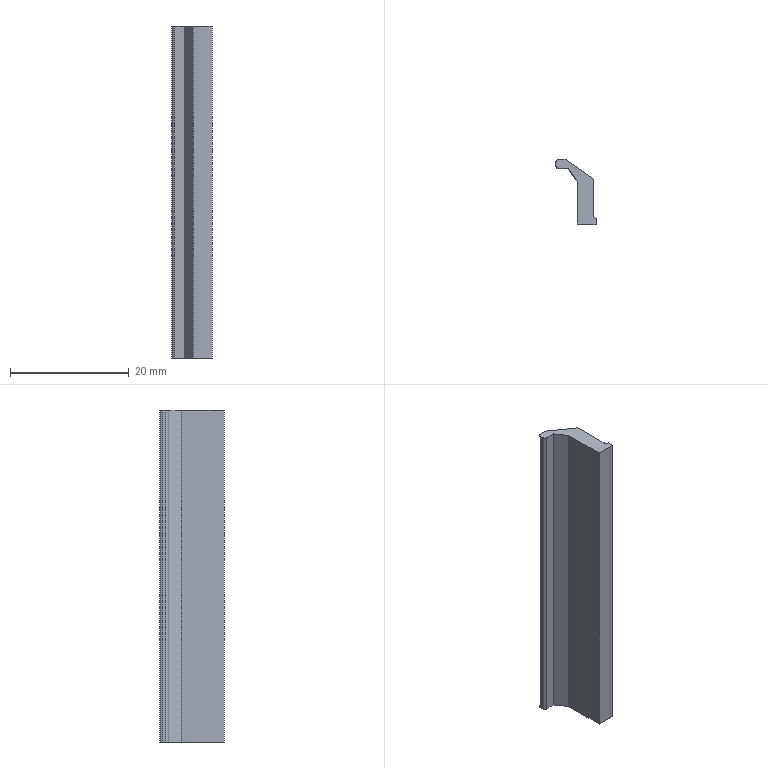Part | NX | features BREP 2 | 2 solids | 32 faces | box 6.787 x 10.9 x 56 mm | volume 3290 mm3 | plane 22 | cylinder 10 | commonest cylinder face diameters 1 x10
STEP:
#1=CARTESIAN_POINT('',(0.2096,1.761,-4.));
#2=VERTEX_POINT('',#1);
#3=CARTESIAN_POINT('',(0.2096,1.761,52.));
#4=VERTEX_POINT('',#3);
#5=CARTESIAN_POINT('',(0.2096,1.761,0.));
#6=DIRECTION('',(0.,0.,1.));
#7=VECTOR('',#6,1000.);
#8=LINE('',#5,#7);
#9=EDGE_CURVE('',#2,#4,#8,.T.);
#10=ORIENTED_EDGE('',*,*,#9,.F.);
#11=CARTESIAN_POINT('',(0.2096,-5.472,-4.));
#12=VERTEX_POINT('',#11);
#13=CARTESIAN_POINT('',(0.2096,24.029,-4.));
#14=DIRECTION('',(0.,-1.,0.));
#15=VECTOR('',#14,1000.);
#16=LINE('',#13,#15);
#17=EDGE_CURVE('',#2,#12,#16,.T.);
#18=ORIENTED_EDGE('',*,*,#17,.T.);
#19=CARTESIAN_POINT('',(0.2096,-5.472,52.));
#20=VERTEX_POINT('',#19);
#21=CARTESIAN_POINT('',(0.2096,-5.472,0.));
#22=DIRECTION('',(0.,0.,1.));
#23=VECTOR('',#22,1000.);
#24=LINE('',#21,#23);
#25=EDGE_CURVE('',#12,#20,#24,.T.);
#26=ORIENTED_EDGE('',*,*,#25,.T.);
#27=CARTESIAN_POINT('',(0.2096,24.029,52.));
#28=DIRECTION('',(0.,-1.,0.));
#29=VECTOR('',#28,1000.);
#30=LINE('',#27,#29);
#31=EDGE_CURVE('',#4,#20,#30,.T.);
#32=ORIENTED_EDGE('',*,*,#31,.F.);
#33=EDGE_LOOP('',(#10,#18,#26,#32));
#34=FACE_BOUND('',#33,.T.);
#35=CARTESIAN_POINT('',(0.2096,-4.473,0.));
#36=DIRECTION('',(1.,0.,0.));
#37=DIRECTION('',(0.,-1.,0.));
#38=AXIS2_PLACEMENT_3D('',#35,#36,#37);
#39=PLANE('',#38);
#40=ADVANCED_FACE('',(#34),#39,.F.);
#41=ORIENTED_EDGE('',*,*,#9,.T.);
#42=CARTESIAN_POINT('',(-1.308,3.928,52.));
#43=VERTEX_POINT('',#42);
#44=CARTESIAN_POINT('',(0.2096,1.761,52.));
#45=DIRECTION('',(0.5736,-0.8192,0.));
#46=VECTOR('',#45,1000.);
#47=LINE('',#44,#46);
#48=EDGE_CURVE('',#43,#4,#47,.T.);
#49=ORIENTED_EDGE('',*,*,#48,.F.);
#50=CARTESIAN_POINT('',(-1.308,3.928,-4.));
#51=VERTEX_POINT('',#50);
#52=CARTESIAN_POINT('',(-1.308,3.928,0.));
#53=DIRECTION('',(0.,0.,1.));
#54=VECTOR('',#53,1000.);
#55=LINE('',#52,#54);
#56=EDGE_CURVE('',#51,#43,#55,.T.);
#57=ORIENTED_EDGE('',*,*,#56,.F.);
#58=CARTESIAN_POINT('',(0.2096,1.761,-4.));
#59=DIRECTION('',(0.5736,-0.8192,0.));
#60=VECTOR('',#59,1000.);
#61=LINE('',#58,#60);
#62=EDGE_CURVE('',#51,#2,#61,.T.);
#63=ORIENTED_EDGE('',*,*,#62,.T.);
#64=EDGE_LOOP('',(#41,#49,#57,#63));
#65=FACE_BOUND('',#64,.T.);
#66=CARTESIAN_POINT('',(0.2096,1.761,0.));
#67=DIRECTION('',(0.8192,0.5736,0.));
#68=DIRECTION('',(0.5736,-0.8192,0.));
#69=AXIS2_PLACEMENT_3D('',#66,#67,#68);
#70=PLANE('',#69);
#71=ADVANCED_FACE('',(#65),#70,.F.);
#72=CARTESIAN_POINT('',(-2.894,3.928,-4.));
#73=VERTEX_POINT('',#72);
#74=CARTESIAN_POINT('',(-2.894,3.928,52.));
#75=VERTEX_POINT('',#74);
#76=CARTESIAN_POINT('',(-2.894,3.928,0.));
#77=DIRECTION('',(0.,0.,1.));
#78=VECTOR('',#77,1000.);
#79=LINE('',#76,#78);
#80=EDGE_CURVE('',#73,#75,#79,.T.);
#81=ORIENTED_EDGE('',*,*,#80,.F.);
#82=CARTESIAN_POINT('',(2.18,3.928,-4.));
#83=DIRECTION('',(1.,0.,0.));
#84=VECTOR('',#83,1000.);
#85=LINE('',#82,#84);
#86=EDGE_CURVE('',#73,#51,#85,.T.);
#87=ORIENTED_EDGE('',*,*,#86,.T.);
#88=ORIENTED_EDGE('',*,*,#56,.T.);
#89=CARTESIAN_POINT('',(2.18,3.928,52.));
#90=DIRECTION('',(1.,0.,0.));
#91=VECTOR('',#90,1000.);
#92=LINE('',#89,#91);
#93=EDGE_CURVE('',#75,#43,#92,.T.);
#94=ORIENTED_EDGE('',*,*,#93,.F.);
#95=EDGE_LOOP('',(#81,#87,#88,#94));
#96=FACE_BOUND('',#95,.T.);
#97=CARTESIAN_POINT('',(-2.694,3.928,0.));
#98=DIRECTION('',(0.,1.,0.));
#99=DIRECTION('',(1.,0.,0.));
#100=AXIS2_PLACEMENT_3D('',#97,#98,#99);
#101=PLANE('',#100);
#102=ADVANCED_FACE('',(#96),#101,.F.);
#103=ORIENTED_EDGE('',*,*,#80,.T.);
#104=CARTESIAN_POINT('',(-3.394,4.428,52.));
#105=VERTEX_POINT('',#104);
#106=CARTESIAN_POINT('',(-2.894,4.428,52.));
#107=DIRECTION('',(0.,0.,1.));
#108=DIRECTION('',(1.,0.,0.));
#109=AXIS2_PLACEMENT_3D('',#106,#107,#108);
#110=CIRCLE('',#109,0.5);
#111=EDGE_CURVE('',#105,#75,#110,.T.);
#112=ORIENTED_EDGE('',*,*,#111,.F.);
#113=CARTESIAN_POINT('',(-3.394,4.428,-4.));
#114=VERTEX_POINT('',#113);
#115=CARTESIAN_POINT('',(-3.394,4.428,0.));
#116=DIRECTION('',(0.,0.,1.));
#117=VECTOR('',#116,1000.);
#118=LINE('',#115,#117);
#119=EDGE_CURVE('',#114,#105,#118,.T.);
#120=ORIENTED_EDGE('',*,*,#119,.F.);
#121=CARTESIAN_POINT('',(-2.894,4.428,-4.));
#122=DIRECTION('',(0.,0.,1.));
#123=DIRECTION('',(1.,0.,0.));
#124=AXIS2_PLACEMENT_3D('',#121,#122,#123);
#125=CIRCLE('',#124,0.5);
#126=EDGE_CURVE('',#114,#73,#125,.T.);
#127=ORIENTED_EDGE('',*,*,#126,.T.);
#128=EDGE_LOOP('',(#103,#112,#120,#127));
#129=FACE_BOUND('',#128,.T.);
#130=CARTESIAN_POINT('',(-2.894,4.428,0.));
#131=DIRECTION('',(0.,0.,1.));
#132=DIRECTION('',(-1.,0.,0.));
#133=AXIS2_PLACEMENT_3D('',#130,#131,#132);
#134=CYLINDRICAL_SURFACE('',#133,0.5);
#135=ADVANCED_FACE('',(#129),#134,.T.);
#136=ORIENTED_EDGE('',*,*,#119,.T.);
#137=CARTESIAN_POINT('',(-3.394,4.928,52.));
#138=VERTEX_POINT('',#137);
#139=CARTESIAN_POINT('',(-3.394,24.029,52.));
#140=DIRECTION('',(0.,-1.,0.));
#141=VECTOR('',#140,1000.);
#142=LINE('',#139,#141);
#143=EDGE_CURVE('',#138,#105,#142,.T.);
#144=ORIENTED_EDGE('',*,*,#143,.F.);
#145=CARTESIAN_POINT('',(-3.394,4.928,-4.));
#146=VERTEX_POINT('',#145);
#147=CARTESIAN_POINT('',(-3.394,4.928,0.));
#148=DIRECTION('',(0.,0.,1.));
#149=VECTOR('',#148,1000.);
#150=LINE('',#147,#149);
#151=EDGE_CURVE('',#146,#138,#150,.T.);
#152=ORIENTED_EDGE('',*,*,#151,.F.);
#153=CARTESIAN_POINT('',(-3.394,24.029,-4.));
#154=DIRECTION('',(0.,-1.,0.));
#155=VECTOR('',#154,1000.);
#156=LINE('',#153,#155);
#157=EDGE_CURVE('',#146,#114,#156,.T.);
#158=ORIENTED_EDGE('',*,*,#157,.T.);
#159=EDGE_LOOP('',(#136,#144,#152,#158));
#160=FACE_BOUND('',#159,.T.);
#161=CARTESIAN_POINT('',(-3.394,4.428,0.));
#162=DIRECTION('',(1.,0.,0.));
#163=DIRECTION('',(0.,-1.,0.));
#164=AXIS2_PLACEMENT_3D('',#161,#162,#163);
#165=PLANE('',#164);
#166=ADVANCED_FACE('',(#160),#165,.F.);
#167=ORIENTED_EDGE('',*,*,#151,.T.);
#168=CARTESIAN_POINT('',(-2.894,5.428,52.));
#169=VERTEX_POINT('',#168);
#170=CARTESIAN_POINT('',(-2.894,4.928,52.));
#171=DIRECTION('',(0.,0.,1.));
#172=DIRECTION('',(1.,0.,0.));
#173=AXIS2_PLACEMENT_3D('',#170,#171,#172);
#174=CIRCLE('',#173,0.5);
#175=EDGE_CURVE('',#169,#138,#174,.T.);
#176=ORIENTED_EDGE('',*,*,#175,.F.);
#177=CARTESIAN_POINT('',(-2.894,5.428,-4.));
#178=VERTEX_POINT('',#177);
#179=CARTESIAN_POINT('',(-2.894,5.427,0.));
#180=DIRECTION('',(0.,0.,1.));
#181=VECTOR('',#180,1000.);
#182=LINE('',#179,#181);
#183=EDGE_CURVE('',#178,#169,#182,.T.);
#184=ORIENTED_EDGE('',*,*,#183,.F.);
#185=CARTESIAN_POINT('',(-2.894,4.928,-4.));
#186=DIRECTION('',(0.,0.,1.));
#187=DIRECTION('',(1.,0.,0.));
#188=AXIS2_PLACEMENT_3D('',#185,#186,#187);
#189=CIRCLE('',#188,0.5);
#190=EDGE_CURVE('',#178,#146,#189,.T.);
#191=ORIENTED_EDGE('',*,*,#190,.T.);
#192=EDGE_LOOP('',(#167,#176,#184,#191));
#193=FACE_BOUND('',#192,.T.);
#194=CARTESIAN_POINT('',(-2.894,4.928,0.));
#195=DIRECTION('',(0.,0.,1.));
#196=DIRECTION('',(-1.,0.,0.));
#197=AXIS2_PLACEMENT_3D('',#194,#195,#196);
#198=CYLINDRICAL_SURFACE('',#197,0.5);
#199=ADVANCED_FACE('',(#193),#198,.T.);
#200=ORIENTED_EDGE('',*,*,#183,.T.);
#201=CARTESIAN_POINT('',(-1.851,5.428,52.));
#202=VERTEX_POINT('',#201);
#203=CARTESIAN_POINT('',(2.18,5.427,52.));
#204=DIRECTION('',(-1.,0.,0.));
#205=VECTOR('',#204,1000.);
#206=LINE('',#203,#205);
#207=EDGE_CURVE('',#202,#169,#206,.T.);
#208=ORIENTED_EDGE('',*,*,#207,.F.);
#209=CARTESIAN_POINT('',(-1.851,5.428,-4.));
#210=VERTEX_POINT('',#209);
#211=CARTESIAN_POINT('',(-1.851,5.428,0.));
#212=DIRECTION('',(0.,0.,1.));
#213=VECTOR('',#212,1000.);
#214=LINE('',#211,#213);
#215=EDGE_CURVE('',#210,#202,#214,.T.);
#216=ORIENTED_EDGE('',*,*,#215,.F.);
#217=CARTESIAN_POINT('',(2.18,5.427,-4.));
#218=DIRECTION('',(-1.,0.,0.));
#219=VECTOR('',#218,1000.);
#220=LINE('',#217,#219);
#221=EDGE_CURVE('',#210,#178,#220,.T.);
#222=ORIENTED_EDGE('',*,*,#221,.T.);
#223=EDGE_LOOP('',(#200,#208,#216,#222));
#224=FACE_BOUND('',#223,.T.);
#225=CARTESIAN_POINT('',(-2.894,5.427,0.));
#226=DIRECTION('',(0.,-1.,0.));
#227=DIRECTION('',(-1.,0.,0.));
#228=AXIS2_PLACEMENT_3D('',#225,#226,#227);
#229=PLANE('',#228);
#230=ADVANCED_FACE('',(#224),#229,.F.);
#231=ORIENTED_EDGE('',*,*,#215,.T.);
#232=CARTESIAN_POINT('',(-1.564,5.337,52.));
#233=VERTEX_POINT('',#232);
#234=CARTESIAN_POINT('',(-1.851,4.928,52.));
#235=DIRECTION('',(0.,0.,1.));
#236=DIRECTION('',(1.,0.,0.));
#237=AXIS2_PLACEMENT_3D('',#234,#235,#236);
#238=CIRCLE('',#237,0.5);
#239=EDGE_CURVE('',#233,#202,#238,.T.);
#240=ORIENTED_EDGE('',*,*,#239,.F.);
#241=CARTESIAN_POINT('',(-1.564,5.337,-4.));
#242=VERTEX_POINT('',#241);
#243=CARTESIAN_POINT('',(-1.564,5.337,0.));
#244=DIRECTION('',(0.,0.,1.));
#245=VECTOR('',#244,1000.);
#246=LINE('',#243,#245);
#247=EDGE_CURVE('',#242,#233,#246,.T.);
#248=ORIENTED_EDGE('',*,*,#247,.F.);
#249=CARTESIAN_POINT('',(-1.851,4.928,-4.));
#250=DIRECTION('',(0.,0.,1.));
#251=DIRECTION('',(1.,0.,0.));
#252=AXIS2_PLACEMENT_3D('',#249,#250,#251);
#253=CIRCLE('',#252,0.5);
#254=EDGE_CURVE('',#242,#210,#253,.T.);
#255=ORIENTED_EDGE('',*,*,#254,.T.);
#256=EDGE_LOOP('',(#231,#240,#248,#255));
#257=FACE_BOUND('',#256,.T.);
#258=CARTESIAN_POINT('',(-1.851,4.928,0.));
#259=DIRECTION('',(0.,0.,1.));
#260=DIRECTION('',(-1.,0.,0.));
#261=AXIS2_PLACEMENT_3D('',#258,#259,#260);
#262=CYLINDRICAL_SURFACE('',#261,0.5);
#263=ADVANCED_FACE('',(#257),#262,.T.);
#264=ORIENTED_EDGE('',*,*,#247,.T.);
#265=CARTESIAN_POINT('',(2.68,2.365,52.));
#266=VERTEX_POINT('',#265);
#267=CARTESIAN_POINT('',(-1.564,5.337,52.));
#268=DIRECTION('',(-0.8192,0.5736,0.));
#269=VECTOR('',#268,1000.);
#270=LINE('',#267,#269);
#271=EDGE_CURVE('',#266,#233,#270,.T.);
#272=ORIENTED_EDGE('',*,*,#271,.F.);
#273=CARTESIAN_POINT('',(2.68,2.365,-4.));
#274=VERTEX_POINT('',#273);
#275=CARTESIAN_POINT('',(2.68,2.365,0.));
#276=DIRECTION('',(0.,0.,1.));
#277=VECTOR('',#276,1000.);
#278=LINE('',#275,#277);
#279=EDGE_CURVE('',#274,#266,#278,.T.);
#280=ORIENTED_EDGE('',*,*,#279,.F.);
#281=CARTESIAN_POINT('',(-1.564,5.337,-4.));
#282=DIRECTION('',(-0.8192,0.5736,0.));
#283=VECTOR('',#282,1000.);
#284=LINE('',#281,#283);
#285=EDGE_CURVE('',#274,#242,#284,.T.);
#286=ORIENTED_EDGE('',*,*,#285,.T.);
#287=EDGE_LOOP('',(#264,#272,#280,#286));
#288=FACE_BOUND('',#287,.T.);
#289=CARTESIAN_POINT('',(-1.564,5.337,0.));
#290=DIRECTION('',(-0.5736,-0.8192,0.));
#291=DIRECTION('',(-0.8192,0.5736,0.));
#292=AXIS2_PLACEMENT_3D('',#289,#290,#291);
#293=PLANE('',#292);
#294=ADVANCED_FACE('',(#288),#293,.F.);
#295=ORIENTED_EDGE('',*,*,#279,.T.);
#296=CARTESIAN_POINT('',(2.894,1.955,52.));
#297=VERTEX_POINT('',#296);
#298=CARTESIAN_POINT('',(2.394,1.955,52.));
#299=DIRECTION('',(0.,0.,1.));
#300=DIRECTION('',(1.,0.,0.));
#301=AXIS2_PLACEMENT_3D('',#298,#299,#300);
#302=CIRCLE('',#301,0.5);
#303=EDGE_CURVE('',#297,#266,#302,.T.);
#304=ORIENTED_EDGE('',*,*,#303,.F.);
#305=CARTESIAN_POINT('',(2.894,1.955,-4.));
#306=VERTEX_POINT('',#305);
#307=CARTESIAN_POINT('',(2.894,1.955,0.));
#308=DIRECTION('',(0.,0.,1.));
#309=VECTOR('',#308,1000.);
#310=LINE('',#307,#309);
#311=EDGE_CURVE('',#306,#297,#310,.T.);
#312=ORIENTED_EDGE('',*,*,#311,.F.);
#313=CARTESIAN_POINT('',(2.394,1.955,-4.));
#314=DIRECTION('',(0.,0.,1.));
#315=DIRECTION('',(1.,0.,0.));
#316=AXIS2_PLACEMENT_3D('',#313,#314,#315);
#317=CIRCLE('',#316,0.5);
#318=EDGE_CURVE('',#306,#274,#317,.T.);
#319=ORIENTED_EDGE('',*,*,#318,.T.);
#320=EDGE_LOOP('',(#295,#304,#312,#319));
#321=FACE_BOUND('',#320,.T.);
#322=CARTESIAN_POINT('',(2.394,1.955,0.));
#323=DIRECTION('',(0.,0.,1.));
#324=DIRECTION('',(-1.,0.,0.));
#325=AXIS2_PLACEMENT_3D('',#322,#323,#324);
#326=CYLINDRICAL_SURFACE('',#325,0.5);
#327=ADVANCED_FACE('',(#321),#326,.T.);
#328=ORIENTED_EDGE('',*,*,#311,.T.);
#329=CARTESIAN_POINT('',(2.894,-3.973,52.));
#330=VERTEX_POINT('',#329);
#331=CARTESIAN_POINT('',(2.894,24.029,52.));
#332=DIRECTION('',(0.,1.,0.));
#333=VECTOR('',#332,1000.);
#334=LINE('',#331,#333);
#335=EDGE_CURVE('',#330,#297,#334,.T.);
#336=ORIENTED_EDGE('',*,*,#335,.F.);
#337=CARTESIAN_POINT('',(2.894,-3.973,-4.));
#338=VERTEX_POINT('',#337);
#339=CARTESIAN_POINT('',(2.894,-3.973,0.));
#340=DIRECTION('',(0.,0.,1.));
#341=VECTOR('',#340,1000.);
#342=LINE('',#339,#341);
#343=EDGE_CURVE('',#338,#330,#342,.T.);
#344=ORIENTED_EDGE('',*,*,#343,.F.);
#345=CARTESIAN_POINT('',(2.894,24.029,-4.));
#346=DIRECTION('',(0.,1.,0.));
#347=VECTOR('',#346,1000.);
#348=LINE('',#345,#347);
#349=EDGE_CURVE('',#338,#306,#348,.T.);
#350=ORIENTED_EDGE('',*,*,#349,.T.);
#351=EDGE_LOOP('',(#328,#336,#344,#350));
#352=FACE_BOUND('',#351,.T.);
#353=CARTESIAN_POINT('',(2.894,1.955,0.));
#354=DIRECTION('',(-1.,0.,0.));
#355=DIRECTION('',(0.,1.,0.));
#356=AXIS2_PLACEMENT_3D('',#353,#354,#355);
#357=PLANE('',#356);
#358=ADVANCED_FACE('',(#352),#357,.F.);
#359=ORIENTED_EDGE('',*,*,#343,.T.);
#360=CARTESIAN_POINT('',(3.394,-4.473,52.));
#361=VERTEX_POINT('',#360);
#362=CARTESIAN_POINT('',(3.394,-3.973,52.));
#363=DIRECTION('',(0.,0.,-1.));
#364=DIRECTION('',(1.,0.,0.));
#365=AXIS2_PLACEMENT_3D('',#362,#363,#364);
#366=CIRCLE('',#365,0.5);
#367=EDGE_CURVE('',#361,#330,#366,.T.);
#368=ORIENTED_EDGE('',*,*,#367,.F.);
#369=CARTESIAN_POINT('',(3.394,-4.473,-4.));
#370=VERTEX_POINT('',#369);
#371=CARTESIAN_POINT('',(3.394,-4.473,0.));
#372=DIRECTION('',(0.,0.,1.));
#373=VECTOR('',#372,1000.);
#374=LINE('',#371,#373);
#375=EDGE_CURVE('',#370,#361,#374,.T.);
#376=ORIENTED_EDGE('',*,*,#375,.F.);
#377=CARTESIAN_POINT('',(3.394,-3.973,-4.));
#378=DIRECTION('',(0.,0.,-1.));
#379=DIRECTION('',(1.,0.,0.));
#380=AXIS2_PLACEMENT_3D('',#377,#378,#379);
#381=CIRCLE('',#380,0.5);
#382=EDGE_CURVE('',#370,#338,#381,.T.);
#383=ORIENTED_EDGE('',*,*,#382,.T.);
#384=EDGE_LOOP('',(#359,#368,#376,#383));
#385=FACE_BOUND('',#384,.T.);
#386=CARTESIAN_POINT('',(3.394,-3.973,0.));
#387=DIRECTION('',(0.,0.,1.));
#388=DIRECTION('',(-1.,0.,0.));
#389=AXIS2_PLACEMENT_3D('',#386,#387,#388);
#390=CYLINDRICAL_SURFACE('',#389,0.5);
#391=ADVANCED_FACE('',(#385),#390,.F.);
#392=ORIENTED_EDGE('',*,*,#375,.T.);
#393=CARTESIAN_POINT('',(3.394,-5.472,52.));
#394=VERTEX_POINT('',#393);
#395=CARTESIAN_POINT('',(3.394,24.029,52.));
#396=DIRECTION('',(0.,1.,0.));
#397=VECTOR('',#396,1000.);
#398=LINE('',#395,#397);
#399=EDGE_CURVE('',#394,#361,#398,.T.);
#400=ORIENTED_EDGE('',*,*,#399,.F.);
#401=CARTESIAN_POINT('',(3.394,-5.472,-4.));
#402=VERTEX_POINT('',#401);
#403=CARTESIAN_POINT('',(3.394,-5.473,0.));
#404=DIRECTION('',(0.,0.,1.));
#405=VECTOR('',#404,1000.);
#406=LINE('',#403,#405);
#407=EDGE_CURVE('',#402,#394,#406,.T.);
#408=ORIENTED_EDGE('',*,*,#407,.F.);
#409=CARTESIAN_POINT('',(3.394,24.029,-4.));
#410=DIRECTION('',(0.,1.,0.));
#411=VECTOR('',#410,1000.);
#412=LINE('',#409,#411);
#413=EDGE_CURVE('',#402,#370,#412,.T.);
#414=ORIENTED_EDGE('',*,*,#413,.T.);
#415=EDGE_LOOP('',(#392,#400,#408,#414));
#416=FACE_BOUND('',#415,.T.);
#417=CARTESIAN_POINT('',(3.394,-4.473,0.));
#418=DIRECTION('',(-1.,0.,0.));
#419=DIRECTION('',(0.,1.,0.));
#420=AXIS2_PLACEMENT_3D('',#417,#418,#419);
#421=PLANE('',#420);
#422=ADVANCED_FACE('',(#416),#421,.F.);
#423=CARTESIAN_POINT('',(2.18,-5.472,-4.));
#424=DIRECTION('',(1.,0.,0.));
#425=VECTOR('',#424,1000.);
#426=LINE('',#423,#425);
#427=EDGE_CURVE('',#12,#402,#426,.T.);
#428=ORIENTED_EDGE('',*,*,#427,.T.);
#429=ORIENTED_EDGE('',*,*,#407,.T.);
#430=CARTESIAN_POINT('',(2.18,-5.472,52.));
#431=DIRECTION('',(1.,0.,0.));
#432=VECTOR('',#431,1000.);
#433=LINE('',#430,#432);
#434=EDGE_CURVE('',#20,#394,#433,.T.);
#435=ORIENTED_EDGE('',*,*,#434,.F.);
#436=ORIENTED_EDGE('',*,*,#25,.F.);
#437=EDGE_LOOP('',(#428,#429,#435,#436));
#438=FACE_BOUND('',#437,.T.);
#439=CARTESIAN_POINT('',(0.2096,-5.472,0.));
#440=DIRECTION('',(0.,-1.,0.));
#441=DIRECTION('',(-1.,0.,0.));
#442=AXIS2_PLACEMENT_3D('',#439,#440,#441);
#443=PLANE('',#442);
#444=ADVANCED_FACE('',(#438),#443,.T.);
#445=ORIENTED_EDGE('',*,*,#399,.T.);
#446=ORIENTED_EDGE('',*,*,#367,.T.);
#447=ORIENTED_EDGE('',*,*,#335,.T.);
#448=ORIENTED_EDGE('',*,*,#303,.T.);
#449=ORIENTED_EDGE('',*,*,#271,.T.);
#450=ORIENTED_EDGE('',*,*,#239,.T.);
#451=ORIENTED_EDGE('',*,*,#207,.T.);
#452=ORIENTED_EDGE('',*,*,#175,.T.);
#453=ORIENTED_EDGE('',*,*,#143,.T.);
#454=ORIENTED_EDGE('',*,*,#111,.T.);
#455=ORIENTED_EDGE('',*,*,#93,.T.);
#456=ORIENTED_EDGE('',*,*,#48,.T.);
#457=ORIENTED_EDGE('',*,*,#31,.T.);
#458=ORIENTED_EDGE('',*,*,#434,.T.);
#459=EDGE_LOOP('',(#445,#446,#447,#448,#449,#450,#451,#452,#453,#454,#455,#456,#457,#458));
#460=FACE_BOUND('',#459,.T.);
#461=CARTESIAN_POINT('',(2.18,24.029,52.));
#462=DIRECTION('',(0.,0.,1.));
#463=DIRECTION('',(-1.,0.,0.));
#464=AXIS2_PLACEMENT_3D('',#461,#462,#463);
#465=PLANE('',#464);
#466=ADVANCED_FACE('',(#460),#465,.T.);
#467=ORIENTED_EDGE('',*,*,#413,.F.);
#468=ORIENTED_EDGE('',*,*,#427,.F.);
#469=ORIENTED_EDGE('',*,*,#17,.F.);
#470=ORIENTED_EDGE('',*,*,#62,.F.);
#471=ORIENTED_EDGE('',*,*,#86,.F.);
#472=ORIENTED_EDGE('',*,*,#126,.F.);
#473=ORIENTED_EDGE('',*,*,#157,.F.);
#474=ORIENTED_EDGE('',*,*,#190,.F.);
#475=ORIENTED_EDGE('',*,*,#221,.F.);
#476=ORIENTED_EDGE('',*,*,#254,.F.);
#477=ORIENTED_EDGE('',*,*,#285,.F.);
#478=ORIENTED_EDGE('',*,*,#318,.F.);
#479=ORIENTED_EDGE('',*,*,#349,.F.);
#480=ORIENTED_EDGE('',*,*,#382,.F.);
#481=EDGE_LOOP('',(#467,#468,#469,#470,#471,#472,#473,#474,#475,#476,#477,#478,#479,#480));
#482=FACE_BOUND('',#481,.T.);
#483=CARTESIAN_POINT('',(2.18,24.029,-4.));
#484=DIRECTION('',(0.,0.,1.));
#485=DIRECTION('',(-1.,0.,0.));
#486=AXIS2_PLACEMENT_3D('',#483,#484,#485);
#487=PLANE('',#486);
#488=ADVANCED_FACE('',(#482),#487,.F.);
#489=CLOSED_SHELL('',(#40,#71,#102,#135,#166,#199,#230,#263,#294,#327,#358,#391,#422,#444,#466,#488));
#490=MANIFOLD_SOLID_BREP('',#489);
#491=CARTESIAN_POINT('',(0.2096,1.761,-4.));
#492=VERTEX_POINT('',#491);
#493=CARTESIAN_POINT('',(0.2096,1.761,52.));
#494=VERTEX_POINT('',#493);
#495=CARTESIAN_POINT('',(0.2096,1.761,0.));
#496=DIRECTION('',(0.,0.,1.));
#497=VECTOR('',#496,1000.);
#498=LINE('',#495,#497);
#499=EDGE_CURVE('',#492,#494,#498,.T.);
#500=ORIENTED_EDGE('',*,*,#499,.F.);
#501=CARTESIAN_POINT('',(0.2096,-5.472,-4.));
#502=VERTEX_POINT('',#501);
#503=CARTESIAN_POINT('',(0.2096,24.029,-4.));
#504=DIRECTION('',(0.,-1.,0.));
#505=VECTOR('',#504,1000.);
#506=LINE('',#503,#505);
#507=EDGE_CURVE('',#492,#502,#506,.T.);
#508=ORIENTED_EDGE('',*,*,#507,.T.);
#509=CARTESIAN_POINT('',(0.2096,-5.472,52.));
#510=VERTEX_POINT('',#509);
#511=CARTESIAN_POINT('',(0.2096,-5.472,0.));
#512=DIRECTION('',(0.,0.,1.));
#513=VECTOR('',#512,1000.);
#514=LINE('',#511,#513);
#515=EDGE_CURVE('',#502,#510,#514,.T.);
#516=ORIENTED_EDGE('',*,*,#515,.T.);
#517=CARTESIAN_POINT('',(0.2096,24.029,52.));
#518=DIRECTION('',(0.,-1.,0.));
#519=VECTOR('',#518,1000.);
#520=LINE('',#517,#519);
#521=EDGE_CURVE('',#494,#510,#520,.T.);
#522=ORIENTED_EDGE('',*,*,#521,.F.);
#523=EDGE_LOOP('',(#500,#508,#516,#522));
#524=FACE_BOUND('',#523,.T.);
#525=CARTESIAN_POINT('',(0.2096,-4.473,0.));
#526=DIRECTION('',(1.,0.,0.));
#527=DIRECTION('',(0.,-1.,0.));
#528=AXIS2_PLACEMENT_3D('',#525,#526,#527);
#529=PLANE('',#528);
#530=ADVANCED_FACE('',(#524),#529,.F.);
#531=ORIENTED_EDGE('',*,*,#499,.T.);
#532=CARTESIAN_POINT('',(-1.308,3.928,52.));
#533=VERTEX_POINT('',#532);
#534=CARTESIAN_POINT('',(0.2096,1.761,52.));
#535=DIRECTION('',(0.5736,-0.8192,0.));
#536=VECTOR('',#535,1000.);
#537=LINE('',#534,#536);
#538=EDGE_CURVE('',#533,#494,#537,.T.);
#539=ORIENTED_EDGE('',*,*,#538,.F.);
#540=CARTESIAN_POINT('',(-1.308,3.928,-4.));
#541=VERTEX_POINT('',#540);
#542=CARTESIAN_POINT('',(-1.308,3.928,0.));
#543=DIRECTION('',(0.,0.,1.));
#544=VECTOR('',#543,1000.);
#545=LINE('',#542,#544);
#546=EDGE_CURVE('',#541,#533,#545,.T.);
#547=ORIENTED_EDGE('',*,*,#546,.F.);
#548=CARTESIAN_POINT('',(0.2096,1.761,-4.));
#549=DIRECTION('',(0.5736,-0.8192,0.));
#550=VECTOR('',#549,1000.);
#551=LINE('',#548,#550);
#552=EDGE_CURVE('',#541,#492,#551,.T.);
#553=ORIENTED_EDGE('',*,*,#552,.T.);
#554=EDGE_LOOP('',(#531,#539,#547,#553));
#555=FACE_BOUND('',#554,.T.);
#556=CARTESIAN_POINT('',(0.2096,1.761,0.));
#557=DIRECTION('',(0.8192,0.5736,0.));
#558=DIRECTION('',(0.5736,-0.8192,0.));
#559=AXIS2_PLACEMENT_3D('',#556,#557,#558);
#560=PLANE('',#559);
#561=ADVANCED_FACE('',(#555),#560,.F.);
#562=CARTESIAN_POINT('',(-2.894,3.928,-4.));
#563=VERTEX_POINT('',#562);
#564=CARTESIAN_POINT('',(-2.894,3.928,52.));
#565=VERTEX_POINT('',#564);
#566=CARTESIAN_POINT('',(-2.894,3.928,0.));
#567=DIRECTION('',(0.,0.,1.));
#568=VECTOR('',#567,1000.);
#569=LINE('',#566,#568);
#570=EDGE_CURVE('',#563,#565,#569,.T.);
#571=ORIENTED_EDGE('',*,*,#570,.F.);
#572=CARTESIAN_POINT('',(2.18,3.928,-4.));
#573=DIRECTION('',(1.,0.,0.));
#574=VECTOR('',#573,1000.);
#575=LINE('',#572,#574);
#576=EDGE_CURVE('',#563,#541,#575,.T.);
#577=ORIENTED_EDGE('',*,*,#576,.T.);
#578=ORIENTED_EDGE('',*,*,#546,.T.);
#579=CARTESIAN_POINT('',(2.18,3.928,52.));
#580=DIRECTION('',(1.,0.,0.));
#581=VECTOR('',#580,1000.);
#582=LINE('',#579,#581);
#583=EDGE_CURVE('',#565,#533,#582,.T.);
#584=ORIENTED_EDGE('',*,*,#583,.F.);
#585=EDGE_LOOP('',(#571,#577,#578,#584));
#586=FACE_BOUND('',#585,.T.);
#587=CARTESIAN_POINT('',(-2.694,3.928,0.));
#588=DIRECTION('',(0.,1.,0.));
#589=DIRECTION('',(1.,0.,0.));
#590=AXIS2_PLACEMENT_3D('',#587,#588,#589);
#591=PLANE('',#590);
#592=ADVANCED_FACE('',(#586),#591,.F.);
#593=ORIENTED_EDGE('',*,*,#570,.T.);
#594=CARTESIAN_POINT('',(-3.394,4.428,52.));
#595=VERTEX_POINT('',#594);
#596=CARTESIAN_POINT('',(-2.894,4.428,52.));
#597=DIRECTION('',(0.,0.,1.));
#598=DIRECTION('',(1.,0.,0.));
#599=AXIS2_PLACEMENT_3D('',#596,#597,#598);
#600=CIRCLE('',#599,0.5);
#601=EDGE_CURVE('',#595,#565,#600,.T.);
#602=ORIENTED_EDGE('',*,*,#601,.F.);
#603=CARTESIAN_POINT('',(-3.394,4.428,-4.));
#604=VERTEX_POINT('',#603);
#605=CARTESIAN_POINT('',(-3.394,4.428,0.));
#606=DIRECTION('',(0.,0.,1.));
#607=VECTOR('',#606,1000.);
#608=LINE('',#605,#607);
#609=EDGE_CURVE('',#604,#595,#608,.T.);
#610=ORIENTED_EDGE('',*,*,#609,.F.);
#611=CARTESIAN_POINT('',(-2.894,4.428,-4.));
#612=DIRECTION('',(0.,0.,1.));
#613=DIRECTION('',(1.,0.,0.));
#614=AXIS2_PLACEMENT_3D('',#611,#612,#613);
#615=CIRCLE('',#614,0.5);
#616=EDGE_CURVE('',#604,#563,#615,.T.);
#617=ORIENTED_EDGE('',*,*,#616,.T.);
#618=EDGE_LOOP('',(#593,#602,#610,#617));
#619=FACE_BOUND('',#618,.T.);
#620=CARTESIAN_POINT('',(-2.894,4.428,0.));
#621=DIRECTION('',(0.,0.,1.));
#622=DIRECTION('',(-1.,0.,0.));
#623=AXIS2_PLACEMENT_3D('',#620,#621,#622);
#624=CYLINDRICAL_SURFACE('',#623,0.5);
#625=ADVANCED_FACE('',(#619),#624,.T.);
#626=ORIENTED_EDGE('',*,*,#609,.T.);
#627=CARTESIAN_POINT('',(-3.394,4.928,52.));
#628=VERTEX_POINT('',#627);
#629=CARTESIAN_POINT('',(-3.394,24.029,52.));
#630=DIRECTION('',(0.,-1.,0.));
#631=VECTOR('',#630,1000.);
#632=LINE('',#629,#631);
#633=EDGE_CURVE('',#628,#595,#632,.T.);
#634=ORIENTED_EDGE('',*,*,#633,.F.);
#635=CARTESIAN_POINT('',(-3.394,4.928,-4.));
#636=VERTEX_POINT('',#635);
#637=CARTESIAN_POINT('',(-3.394,4.928,0.));
#638=DIRECTION('',(0.,0.,1.));
#639=VECTOR('',#638,1000.);
#640=LINE('',#637,#639);
#641=EDGE_CURVE('',#636,#628,#640,.T.);
#642=ORIENTED_EDGE('',*,*,#641,.F.);
#643=CARTESIAN_POINT('',(-3.394,24.029,-4.));
#644=DIRECTION('',(0.,-1.,0.));
#645=VECTOR('',#644,1000.);
#646=LINE('',#643,#645);
#647=EDGE_CURVE('',#636,#604,#646,.T.);
#648=ORIENTED_EDGE('',*,*,#647,.T.);
#649=EDGE_LOOP('',(#626,#634,#642,#648));
#650=FACE_BOUND('',#649,.T.);
#651=CARTESIAN_POINT('',(-3.394,4.428,0.));
#652=DIRECTION('',(1.,0.,0.));
#653=DIRECTION('',(0.,-1.,0.));
#654=AXIS2_PLACEMENT_3D('',#651,#652,#653);
#655=PLANE('',#654);
#656=ADVANCED_FACE('',(#650),#655,.F.);
#657=ORIENTED_EDGE('',*,*,#641,.T.);
#658=CARTESIAN_POINT('',(-2.894,5.428,52.));
#659=VERTEX_POINT('',#658);
#660=CARTESIAN_POINT('',(-2.894,4.928,52.));
#661=DIRECTION('',(0.,0.,1.));
#662=DIRECTION('',(1.,0.,0.));
#663=AXIS2_PLACEMENT_3D('',#660,#661,#662);
#664=CIRCLE('',#663,0.5);
#665=EDGE_CURVE('',#659,#628,#664,.T.);
#666=ORIENTED_EDGE('',*,*,#665,.F.);
#667=CARTESIAN_POINT('',(-2.894,5.428,-4.));
#668=VERTEX_POINT('',#667);
#669=CARTESIAN_POINT('',(-2.894,5.427,0.));
#670=DIRECTION('',(0.,0.,1.));
#671=VECTOR('',#670,1000.);
#672=LINE('',#669,#671);
#673=EDGE_CURVE('',#668,#659,#672,.T.);
#674=ORIENTED_EDGE('',*,*,#673,.F.);
#675=CARTESIAN_POINT('',(-2.894,4.928,-4.));
#676=DIRECTION('',(0.,0.,1.));
#677=DIRECTION('',(1.,0.,0.));
#678=AXIS2_PLACEMENT_3D('',#675,#676,#677);
#679=CIRCLE('',#678,0.5);
#680=EDGE_CURVE('',#668,#636,#679,.T.);
#681=ORIENTED_EDGE('',*,*,#680,.T.);
#682=EDGE_LOOP('',(#657,#666,#674,#681));
#683=FACE_BOUND('',#682,.T.);
#684=CARTESIAN_POINT('',(-2.894,4.928,0.));
#685=DIRECTION('',(0.,0.,1.));
#686=DIRECTION('',(-1.,0.,0.));
#687=AXIS2_PLACEMENT_3D('',#684,#685,#686);
#688=CYLINDRICAL_SURFACE('',#687,0.5);
#689=ADVANCED_FACE('',(#683),#688,.T.);
#690=ORIENTED_EDGE('',*,*,#673,.T.);
#691=CARTESIAN_POINT('',(-1.851,5.428,52.));
#692=VERTEX_POINT('',#691);
#693=CARTESIAN_POINT('',(2.18,5.427,52.));
#694=DIRECTION('',(-1.,0.,0.));
#695=VECTOR('',#694,1000.);
#696=LINE('',#693,#695);
#697=EDGE_CURVE('',#692,#659,#696,.T.);
#698=ORIENTED_EDGE('',*,*,#697,.F.);
#699=CARTESIAN_POINT('',(-1.851,5.428,-4.));
#700=VERTEX_POINT('',#699);
#701=CARTESIAN_POINT('',(-1.851,5.428,0.));
#702=DIRECTION('',(0.,0.,1.));
#703=VECTOR('',#702,1000.);
#704=LINE('',#701,#703);
#705=EDGE_CURVE('',#700,#692,#704,.T.);
#706=ORIENTED_EDGE('',*,*,#705,.F.);
#707=CARTESIAN_POINT('',(2.18,5.427,-4.));
#708=DIRECTION('',(-1.,0.,0.));
#709=VECTOR('',#708,1000.);
#710=LINE('',#707,#709);
#711=EDGE_CURVE('',#700,#668,#710,.T.);
#712=ORIENTED_EDGE('',*,*,#711,.T.);
#713=EDGE_LOOP('',(#690,#698,#706,#712));
#714=FACE_BOUND('',#713,.T.);
#715=CARTESIAN_POINT('',(-2.894,5.427,0.));
#716=DIRECTION('',(0.,-1.,0.));
#717=DIRECTION('',(-1.,0.,0.));
#718=AXIS2_PLACEMENT_3D('',#715,#716,#717);
#719=PLANE('',#718);
#720=ADVANCED_FACE('',(#714),#719,.F.);
#721=ORIENTED_EDGE('',*,*,#705,.T.);
#722=CARTESIAN_POINT('',(-1.564,5.337,52.));
#723=VERTEX_POINT('',#722);
#724=CARTESIAN_POINT('',(-1.851,4.928,52.));
#725=DIRECTION('',(0.,0.,1.));
#726=DIRECTION('',(1.,0.,0.));
#727=AXIS2_PLACEMENT_3D('',#724,#725,#726);
#728=CIRCLE('',#727,0.5);
#729=EDGE_CURVE('',#723,#692,#728,.T.);
#730=ORIENTED_EDGE('',*,*,#729,.F.);
#731=CARTESIAN_POINT('',(-1.564,5.337,-4.));
#732=VERTEX_POINT('',#731);
#733=CARTESIAN_POINT('',(-1.564,5.337,0.));
#734=DIRECTION('',(0.,0.,1.));
#735=VECTOR('',#734,1000.);
#736=LINE('',#733,#735);
#737=EDGE_CURVE('',#732,#723,#736,.T.);
#738=ORIENTED_EDGE('',*,*,#737,.F.);
#739=CARTESIAN_POINT('',(-1.851,4.928,-4.));
#740=DIRECTION('',(0.,0.,1.));
#741=DIRECTION('',(1.,0.,0.));
#742=AXIS2_PLACEMENT_3D('',#739,#740,#741);
#743=CIRCLE('',#742,0.5);
#744=EDGE_CURVE('',#732,#700,#743,.T.);
#745=ORIENTED_EDGE('',*,*,#744,.T.);
#746=EDGE_LOOP('',(#721,#730,#738,#745));
#747=FACE_BOUND('',#746,.T.);
#748=CARTESIAN_POINT('',(-1.851,4.928,0.));
#749=DIRECTION('',(0.,0.,1.));
#750=DIRECTION('',(-1.,0.,0.));
#751=AXIS2_PLACEMENT_3D('',#748,#749,#750);
#752=CYLINDRICAL_SURFACE('',#751,0.5);
#753=ADVANCED_FACE('',(#747),#752,.T.);
#754=ORIENTED_EDGE('',*,*,#737,.T.);
#755=CARTESIAN_POINT('',(2.68,2.365,52.));
#756=VERTEX_POINT('',#755);
#757=CARTESIAN_POINT('',(-1.564,5.337,52.));
#758=DIRECTION('',(-0.8192,0.5736,0.));
#759=VECTOR('',#758,1000.);
#760=LINE('',#757,#759);
#761=EDGE_CURVE('',#756,#723,#760,.T.);
#762=ORIENTED_EDGE('',*,*,#761,.F.);
#763=CARTESIAN_POINT('',(2.68,2.365,-4.));
#764=VERTEX_POINT('',#763);
#765=CARTESIAN_POINT('',(2.68,2.365,0.));
#766=DIRECTION('',(0.,0.,1.));
#767=VECTOR('',#766,1000.);
#768=LINE('',#765,#767);
#769=EDGE_CURVE('',#764,#756,#768,.T.);
#770=ORIENTED_EDGE('',*,*,#769,.F.);
#771=CARTESIAN_POINT('',(-1.564,5.337,-4.));
#772=DIRECTION('',(-0.8192,0.5736,0.));
#773=VECTOR('',#772,1000.);
#774=LINE('',#771,#773);
#775=EDGE_CURVE('',#764,#732,#774,.T.);
#776=ORIENTED_EDGE('',*,*,#775,.T.);
#777=EDGE_LOOP('',(#754,#762,#770,#776));
#778=FACE_BOUND('',#777,.T.);
#779=CARTESIAN_POINT('',(-1.564,5.337,0.));
#780=DIRECTION('',(-0.5736,-0.8192,0.));
#781=DIRECTION('',(-0.8192,0.5736,0.));
#782=AXIS2_PLACEMENT_3D('',#779,#780,#781);
#783=PLANE('',#782);
#784=ADVANCED_FACE('',(#778),#783,.F.);
#785=ORIENTED_EDGE('',*,*,#769,.T.);
#786=CARTESIAN_POINT('',(2.894,1.955,52.));
#787=VERTEX_POINT('',#786);
#788=CARTESIAN_POINT('',(2.394,1.955,52.));
#789=DIRECTION('',(0.,0.,1.));
#790=DIRECTION('',(1.,0.,0.));
#791=AXIS2_PLACEMENT_3D('',#788,#789,#790);
#792=CIRCLE('',#791,0.5);
#793=EDGE_CURVE('',#787,#756,#792,.T.);
#794=ORIENTED_EDGE('',*,*,#793,.F.);
#795=CARTESIAN_POINT('',(2.894,1.955,-4.));
#796=VERTEX_POINT('',#795);
#797=CARTESIAN_POINT('',(2.894,1.955,0.));
#798=DIRECTION('',(0.,0.,1.));
#799=VECTOR('',#798,1000.);
#800=LINE('',#797,#799);
#801=EDGE_CURVE('',#796,#787,#800,.T.);
#802=ORIENTED_EDGE('',*,*,#801,.F.);
#803=CARTESIAN_POINT('',(2.394,1.955,-4.));
#804=DIRECTION('',(0.,0.,1.));
#805=DIRECTION('',(1.,0.,0.));
#806=AXIS2_PLACEMENT_3D('',#803,#804,#805);
#807=CIRCLE('',#806,0.5);
#808=EDGE_CURVE('',#796,#764,#807,.T.);
#809=ORIENTED_EDGE('',*,*,#808,.T.);
#810=EDGE_LOOP('',(#785,#794,#802,#809));
#811=FACE_BOUND('',#810,.T.);
#812=CARTESIAN_POINT('',(2.394,1.955,0.));
#813=DIRECTION('',(0.,0.,1.));
#814=DIRECTION('',(-1.,0.,0.));
#815=AXIS2_PLACEMENT_3D('',#812,#813,#814);
#816=CYLINDRICAL_SURFACE('',#815,0.5);
#817=ADVANCED_FACE('',(#811),#816,.T.);
#818=ORIENTED_EDGE('',*,*,#801,.T.);
#819=CARTESIAN_POINT('',(2.894,-3.973,52.));
#820=VERTEX_POINT('',#819);
#821=CARTESIAN_POINT('',(2.894,24.029,52.));
#822=DIRECTION('',(0.,1.,0.));
#823=VECTOR('',#822,1000.);
#824=LINE('',#821,#823);
#825=EDGE_CURVE('',#820,#787,#824,.T.);
#826=ORIENTED_EDGE('',*,*,#825,.F.);
#827=CARTESIAN_POINT('',(2.894,-3.973,-4.));
#828=VERTEX_POINT('',#827);
#829=CARTESIAN_POINT('',(2.894,-3.973,0.));
#830=DIRECTION('',(0.,0.,1.));
#831=VECTOR('',#830,1000.);
#832=LINE('',#829,#831);
#833=EDGE_CURVE('',#828,#820,#832,.T.);
#834=ORIENTED_EDGE('',*,*,#833,.F.);
#835=CARTESIAN_POINT('',(2.894,24.029,-4.));
#836=DIRECTION('',(0.,1.,0.));
#837=VECTOR('',#836,1000.);
#838=LINE('',#835,#837);
#839=EDGE_CURVE('',#828,#796,#838,.T.);
#840=ORIENTED_EDGE('',*,*,#839,.T.);
#841=EDGE_LOOP('',(#818,#826,#834,#840));
#842=FACE_BOUND('',#841,.T.);
#843=CARTESIAN_POINT('',(2.894,1.955,0.));
#844=DIRECTION('',(-1.,0.,0.));
#845=DIRECTION('',(0.,1.,0.));
#846=AXIS2_PLACEMENT_3D('',#843,#844,#845);
#847=PLANE('',#846);
#848=ADVANCED_FACE('',(#842),#847,.F.);
#849=ORIENTED_EDGE('',*,*,#833,.T.);
#850=CARTESIAN_POINT('',(3.394,-4.473,52.));
#851=VERTEX_POINT('',#850);
#852=CARTESIAN_POINT('',(3.394,-3.973,52.));
#853=DIRECTION('',(0.,0.,-1.));
#854=DIRECTION('',(1.,0.,0.));
#855=AXIS2_PLACEMENT_3D('',#852,#853,#854);
#856=CIRCLE('',#855,0.5);
#857=EDGE_CURVE('',#851,#820,#856,.T.);
#858=ORIENTED_EDGE('',*,*,#857,.F.);
#859=CARTESIAN_POINT('',(3.394,-4.473,-4.));
#860=VERTEX_POINT('',#859);
#861=CARTESIAN_POINT('',(3.394,-4.473,0.));
#862=DIRECTION('',(0.,0.,1.));
#863=VECTOR('',#862,1000.);
#864=LINE('',#861,#863);
#865=EDGE_CURVE('',#860,#851,#864,.T.);
#866=ORIENTED_EDGE('',*,*,#865,.F.);
#867=CARTESIAN_POINT('',(3.394,-3.973,-4.));
#868=DIRECTION('',(0.,0.,-1.));
#869=DIRECTION('',(1.,0.,0.));
#870=AXIS2_PLACEMENT_3D('',#867,#868,#869);
#871=CIRCLE('',#870,0.5);
#872=EDGE_CURVE('',#860,#828,#871,.T.);
#873=ORIENTED_EDGE('',*,*,#872,.T.);
#874=EDGE_LOOP('',(#849,#858,#866,#873));
#875=FACE_BOUND('',#874,.T.);
#876=CARTESIAN_POINT('',(3.394,-3.973,0.));
#877=DIRECTION('',(0.,0.,1.));
#878=DIRECTION('',(-1.,0.,0.));
#879=AXIS2_PLACEMENT_3D('',#876,#877,#878);
#880=CYLINDRICAL_SURFACE('',#879,0.5);
#881=ADVANCED_FACE('',(#875),#880,.F.);
#882=ORIENTED_EDGE('',*,*,#865,.T.);
#883=CARTESIAN_POINT('',(3.394,-5.472,52.));
#884=VERTEX_POINT('',#883);
#885=CARTESIAN_POINT('',(3.394,24.029,52.));
#886=DIRECTION('',(0.,1.,0.));
#887=VECTOR('',#886,1000.);
#888=LINE('',#885,#887);
#889=EDGE_CURVE('',#884,#851,#888,.T.);
#890=ORIENTED_EDGE('',*,*,#889,.F.);
#891=CARTESIAN_POINT('',(3.394,-5.472,-4.));
#892=VERTEX_POINT('',#891);
#893=CARTESIAN_POINT('',(3.394,-5.473,0.));
#894=DIRECTION('',(0.,0.,1.));
#895=VECTOR('',#894,1000.);
#896=LINE('',#893,#895);
#897=EDGE_CURVE('',#892,#884,#896,.T.);
#898=ORIENTED_EDGE('',*,*,#897,.F.);
#899=CARTESIAN_POINT('',(3.394,24.029,-4.));
#900=DIRECTION('',(0.,1.,0.));
#901=VECTOR('',#900,1000.);
#902=LINE('',#899,#901);
#903=EDGE_CURVE('',#892,#860,#902,.T.);
#904=ORIENTED_EDGE('',*,*,#903,.T.);
#905=EDGE_LOOP('',(#882,#890,#898,#904));
#906=FACE_BOUND('',#905,.T.);
#907=CARTESIAN_POINT('',(3.394,-4.473,0.));
#908=DIRECTION('',(-1.,0.,0.));
#909=DIRECTION('',(0.,1.,0.));
#910=AXIS2_PLACEMENT_3D('',#907,#908,#909);
#911=PLANE('',#910);
#912=ADVANCED_FACE('',(#906),#911,.F.);
#913=CARTESIAN_POINT('',(2.18,-5.472,-4.));
#914=DIRECTION('',(1.,0.,0.));
#915=VECTOR('',#914,1000.);
#916=LINE('',#913,#915);
#917=EDGE_CURVE('',#502,#892,#916,.T.);
#918=ORIENTED_EDGE('',*,*,#917,.T.);
#919=ORIENTED_EDGE('',*,*,#897,.T.);
#920=CARTESIAN_POINT('',(2.18,-5.472,52.));
#921=DIRECTION('',(1.,0.,0.));
#922=VECTOR('',#921,1000.);
#923=LINE('',#920,#922);
#924=EDGE_CURVE('',#510,#884,#923,.T.);
#925=ORIENTED_EDGE('',*,*,#924,.F.);
#926=ORIENTED_EDGE('',*,*,#515,.F.);
#927=EDGE_LOOP('',(#918,#919,#925,#926));
#928=FACE_BOUND('',#927,.T.);
#929=CARTESIAN_POINT('',(0.2096,-5.472,0.));
#930=DIRECTION('',(0.,-1.,0.));
#931=DIRECTION('',(-1.,0.,0.));
#932=AXIS2_PLACEMENT_3D('',#929,#930,#931);
#933=PLANE('',#932);
#934=ADVANCED_FACE('',(#928),#933,.T.);
#935=ORIENTED_EDGE('',*,*,#889,.T.);
#936=ORIENTED_EDGE('',*,*,#857,.T.);
#937=ORIENTED_EDGE('',*,*,#825,.T.);
#938=ORIENTED_EDGE('',*,*,#793,.T.);
#939=ORIENTED_EDGE('',*,*,#761,.T.);
#940=ORIENTED_EDGE('',*,*,#729,.T.);
#941=ORIENTED_EDGE('',*,*,#697,.T.);
#942=ORIENTED_EDGE('',*,*,#665,.T.);
#943=ORIENTED_EDGE('',*,*,#633,.T.);
#944=ORIENTED_EDGE('',*,*,#601,.T.);
#945=ORIENTED_EDGE('',*,*,#583,.T.);
#946=ORIENTED_EDGE('',*,*,#538,.T.);
#947=ORIENTED_EDGE('',*,*,#521,.T.);
#948=ORIENTED_EDGE('',*,*,#924,.T.);
#949=EDGE_LOOP('',(#935,#936,#937,#938,#939,#940,#941,#942,#943,#944,#945,#946,#947,#948));
#950=FACE_BOUND('',#949,.T.);
#951=CARTESIAN_POINT('',(2.18,24.029,52.));
#952=DIRECTION('',(0.,0.,1.));
#953=DIRECTION('',(-1.,0.,0.));
#954=AXIS2_PLACEMENT_3D('',#951,#952,#953);
#955=PLANE('',#954);
#956=ADVANCED_FACE('',(#950),#955,.T.);
#957=ORIENTED_EDGE('',*,*,#903,.F.);
#958=ORIENTED_EDGE('',*,*,#917,.F.);
#959=ORIENTED_EDGE('',*,*,#507,.F.);
#960=ORIENTED_EDGE('',*,*,#552,.F.);
#961=ORIENTED_EDGE('',*,*,#576,.F.);
#962=ORIENTED_EDGE('',*,*,#616,.F.);
#963=ORIENTED_EDGE('',*,*,#647,.F.);
#964=ORIENTED_EDGE('',*,*,#680,.F.);
#965=ORIENTED_EDGE('',*,*,#711,.F.);
#966=ORIENTED_EDGE('',*,*,#744,.F.);
#967=ORIENTED_EDGE('',*,*,#775,.F.);
#968=ORIENTED_EDGE('',*,*,#808,.F.);
#969=ORIENTED_EDGE('',*,*,#839,.F.);
#970=ORIENTED_EDGE('',*,*,#872,.F.);
#971=EDGE_LOOP('',(#957,#958,#959,#960,#961,#962,#963,#964,#965,#966,#967,#968,#969,#970));
#972=FACE_BOUND('',#971,.T.);
#973=CARTESIAN_POINT('',(2.18,24.029,-4.));
#974=DIRECTION('',(0.,0.,1.));
#975=DIRECTION('',(-1.,0.,0.));
#976=AXIS2_PLACEMENT_3D('',#973,#974,#975);
#977=PLANE('',#976);
#978=ADVANCED_FACE('',(#972),#977,.F.);
#979=CLOSED_SHELL('',(#530,#561,#592,#625,#656,#689,#720,#753,#784,#817,#848,#881,#912,#934,#956,#978));
#980=MANIFOLD_SOLID_BREP('',#979);
#981=(LENGTH_UNIT()NAMED_UNIT(*)SI_UNIT(.MILLI.,.METRE.));
#982=UNCERTAINTY_MEASURE_WITH_UNIT(LENGTH_MEASURE(0.00001),#981,'','');
#983=(NAMED_UNIT(*)PLANE_ANGLE_UNIT()SI_UNIT($,.RADIAN.));
#984=(NAMED_UNIT(*)SI_UNIT($,.STERADIAN.)SOLID_ANGLE_UNIT());
#985=(GEOMETRIC_REPRESENTATION_CONTEXT(3)GLOBAL_UNCERTAINTY_ASSIGNED_CONTEXT((#982))GLOBAL_UNIT_ASSIGNED_CONTEXT((#981,#983,#984))REPRESENTATION_CONTEXT('',''));
#986=ADVANCED_BREP_SHAPE_REPRESENTATION('',(#490,#980),#985);